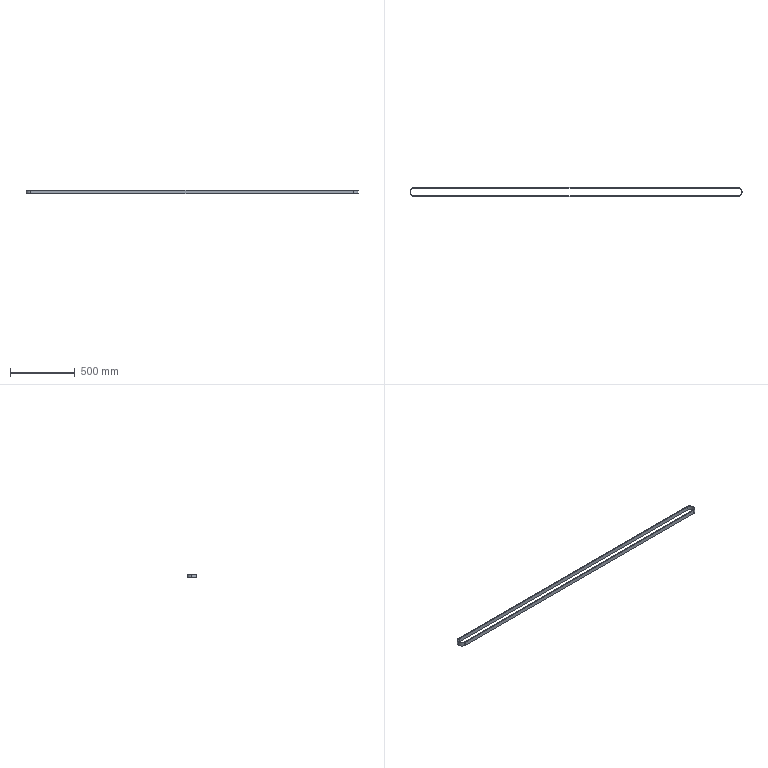Part | SolidWorks | features ExtruThin 1 | 1 solid | 12 faces | box 2564 x 70.66 x 30 mm | volume 701169 mm3 | cylinder 6 | plane 6 | commonest cylinder face diameters 61.66 x3 70.66 x3
STEP:
#1=CARTESIAN_POINT('',(-1246.5,30.83,30.));
#2=VERTEX_POINT('',#1);
#3=CARTESIAN_POINT('',(-1277.33,0.,30.));
#4=VERTEX_POINT('',#3);
#5=CARTESIAN_POINT('',(-1246.5,0.,30.));
#6=DIRECTION('',(0.,0.,1.));
#7=DIRECTION('',(1.,0.,0.));
#8=AXIS2_PLACEMENT_3D('',#5,#6,#7);
#9=CIRCLE('',#8,30.83);
#10=EDGE_CURVE('',#2,#4,#9,.T.);
#11=ORIENTED_EDGE('',*,*,#10,.T.);
#12=CARTESIAN_POINT('',(-1277.33,0.,0.));
#13=VERTEX_POINT('',#12);
#14=CARTESIAN_POINT('',(-1277.33,0.,30.));
#15=DIRECTION('',(0.,0.,-1.));
#16=VECTOR('',#15,1000.);
#17=LINE('',#14,#16);
#18=EDGE_CURVE('',#4,#13,#17,.T.);
#19=ORIENTED_EDGE('',*,*,#18,.T.);
#20=CARTESIAN_POINT('',(-1246.5,30.83,0.));
#21=VERTEX_POINT('',#20);
#22=CARTESIAN_POINT('',(-1246.5,0.,0.));
#23=DIRECTION('',(0.,0.,1.));
#24=DIRECTION('',(1.,0.,0.));
#25=AXIS2_PLACEMENT_3D('',#22,#23,#24);
#26=CIRCLE('',#25,30.83);
#27=EDGE_CURVE('',#21,#13,#26,.T.);
#28=ORIENTED_EDGE('',*,*,#27,.F.);
#29=CARTESIAN_POINT('',(-1246.5,30.83,30.));
#30=DIRECTION('',(0.,0.,-1.));
#31=VECTOR('',#30,1000.);
#32=LINE('',#29,#31);
#33=EDGE_CURVE('',#2,#21,#32,.T.);
#34=ORIENTED_EDGE('',*,*,#33,.F.);
#35=EDGE_LOOP('',(#11,#19,#28,#34));
#36=FACE_OUTER_BOUND('',#35,.T.);
#37=CARTESIAN_POINT('',(-1246.5,0.,30.));
#38=DIRECTION('',(0.,0.,-1.));
#39=DIRECTION('',(-1.,0.,0.));
#40=AXIS2_PLACEMENT_3D('',#37,#38,#39);
#41=CYLINDRICAL_SURFACE('',#40,30.83);
#42=ADVANCED_FACE('',(#36),#41,.F.);
#43=CARTESIAN_POINT('',(-1281.83,0.,30.));
#44=VERTEX_POINT('',#43);
#45=CARTESIAN_POINT('',(-1246.5,-35.33,30.));
#46=VERTEX_POINT('',#45);
#47=CARTESIAN_POINT('',(-1246.5,0.,30.));
#48=DIRECTION('',(0.,0.,1.));
#49=DIRECTION('',(1.,0.,0.));
#50=AXIS2_PLACEMENT_3D('',#47,#48,#49);
#51=CIRCLE('',#50,35.33);
#52=EDGE_CURVE('',#44,#46,#51,.T.);
#53=ORIENTED_EDGE('',*,*,#52,.F.);
#54=CARTESIAN_POINT('',(-1281.83,0.,0.));
#55=VERTEX_POINT('',#54);
#56=CARTESIAN_POINT('',(-1281.83,0.,30.));
#57=DIRECTION('',(0.,0.,-1.));
#58=VECTOR('',#57,1000.);
#59=LINE('',#56,#58);
#60=EDGE_CURVE('',#44,#55,#59,.T.);
#61=ORIENTED_EDGE('',*,*,#60,.T.);
#62=CARTESIAN_POINT('',(-1246.5,-35.33,0.));
#63=VERTEX_POINT('',#62);
#64=CARTESIAN_POINT('',(-1246.5,0.,0.));
#65=DIRECTION('',(0.,0.,1.));
#66=DIRECTION('',(1.,0.,0.));
#67=AXIS2_PLACEMENT_3D('',#64,#65,#66);
#68=CIRCLE('',#67,35.33);
#69=EDGE_CURVE('',#55,#63,#68,.T.);
#70=ORIENTED_EDGE('',*,*,#69,.T.);
#71=CARTESIAN_POINT('',(-1246.5,-35.33,30.));
#72=DIRECTION('',(0.,0.,-1.));
#73=VECTOR('',#72,1000.);
#74=LINE('',#71,#73);
#75=EDGE_CURVE('',#46,#63,#74,.T.);
#76=ORIENTED_EDGE('',*,*,#75,.F.);
#77=EDGE_LOOP('',(#53,#61,#70,#76));
#78=FACE_OUTER_BOUND('',#77,.T.);
#79=CARTESIAN_POINT('',(-1246.5,0.,30.));
#80=DIRECTION('',(0.,0.,-1.));
#81=DIRECTION('',(-1.,0.,0.));
#82=AXIS2_PLACEMENT_3D('',#79,#80,#81);
#83=CYLINDRICAL_SURFACE('',#82,35.33);
#84=ADVANCED_FACE('',(#78),#83,.T.);
#85=CARTESIAN_POINT('',(-1246.5,35.33,30.));
#86=VERTEX_POINT('',#85);
#87=CARTESIAN_POINT('',(-1246.5,0.,30.));
#88=DIRECTION('',(0.,0.,1.));
#89=DIRECTION('',(1.,0.,0.));
#90=AXIS2_PLACEMENT_3D('',#87,#88,#89);
#91=CIRCLE('',#90,35.33);
#92=EDGE_CURVE('',#86,#44,#91,.T.);
#93=ORIENTED_EDGE('',*,*,#92,.T.);
#94=ORIENTED_EDGE('',*,*,#52,.T.);
#95=CARTESIAN_POINT('',(1246.5,-35.33,30.));
#96=VERTEX_POINT('',#95);
#97=CARTESIAN_POINT('',(-1246.5,-35.33,30.));
#98=DIRECTION('',(1.,0.,0.));
#99=VECTOR('',#98,1000.);
#100=LINE('',#97,#99);
#101=EDGE_CURVE('',#46,#96,#100,.T.);
#102=ORIENTED_EDGE('',*,*,#101,.T.);
#103=CARTESIAN_POINT('',(1246.5,35.33,30.));
#104=VERTEX_POINT('',#103);
#105=CARTESIAN_POINT('',(1246.5,0.,30.));
#106=DIRECTION('',(0.,0.,1.));
#107=DIRECTION('',(1.,0.,0.));
#108=AXIS2_PLACEMENT_3D('',#105,#106,#107);
#109=CIRCLE('',#108,35.33);
#110=EDGE_CURVE('',#96,#104,#109,.T.);
#111=ORIENTED_EDGE('',*,*,#110,.T.);
#112=CARTESIAN_POINT('',(-1246.5,35.33,30.));
#113=DIRECTION('',(-1.,0.,0.));
#114=VECTOR('',#113,1000.);
#115=LINE('',#112,#114);
#116=EDGE_CURVE('',#104,#86,#115,.T.);
#117=ORIENTED_EDGE('',*,*,#116,.T.);
#118=EDGE_LOOP('',(#93,#94,#102,#111,#117));
#119=FACE_OUTER_BOUND('',#118,.T.);
#120=CARTESIAN_POINT('',(-1246.5,-30.83,30.));
#121=VERTEX_POINT('',#120);
#122=CARTESIAN_POINT('',(1246.5,-30.83,30.));
#123=VERTEX_POINT('',#122);
#124=CARTESIAN_POINT('',(-1246.5,-30.83,30.));
#125=DIRECTION('',(1.,0.,0.));
#126=VECTOR('',#125,1000.);
#127=LINE('',#124,#126);
#128=EDGE_CURVE('',#121,#123,#127,.T.);
#129=ORIENTED_EDGE('',*,*,#128,.F.);
#130=CARTESIAN_POINT('',(-1246.5,0.,30.));
#131=DIRECTION('',(0.,0.,1.));
#132=DIRECTION('',(1.,0.,0.));
#133=AXIS2_PLACEMENT_3D('',#130,#131,#132);
#134=CIRCLE('',#133,30.83);
#135=EDGE_CURVE('',#4,#121,#134,.T.);
#136=ORIENTED_EDGE('',*,*,#135,.F.);
#137=ORIENTED_EDGE('',*,*,#10,.F.);
#138=CARTESIAN_POINT('',(1246.5,30.83,30.));
#139=VERTEX_POINT('',#138);
#140=CARTESIAN_POINT('',(-1246.5,30.83,30.));
#141=DIRECTION('',(-1.,0.,0.));
#142=VECTOR('',#141,1000.);
#143=LINE('',#140,#142);
#144=EDGE_CURVE('',#139,#2,#143,.T.);
#145=ORIENTED_EDGE('',*,*,#144,.F.);
#146=CARTESIAN_POINT('',(1246.5,0.,30.));
#147=DIRECTION('',(0.,0.,1.));
#148=DIRECTION('',(1.,0.,0.));
#149=AXIS2_PLACEMENT_3D('',#146,#147,#148);
#150=CIRCLE('',#149,30.83);
#151=EDGE_CURVE('',#123,#139,#150,.T.);
#152=ORIENTED_EDGE('',*,*,#151,.F.);
#153=EDGE_LOOP('',(#129,#136,#137,#145,#152));
#154=FACE_BOUND('',#153,.T.);
#155=CARTESIAN_POINT('',(-1246.5,0.,30.));
#156=DIRECTION('',(0.,0.,1.));
#157=DIRECTION('',(1.,0.,0.));
#158=AXIS2_PLACEMENT_3D('',#155,#156,#157);
#159=PLANE('',#158);
#160=ADVANCED_FACE('',(#119,#154),#159,.T.);
#161=CARTESIAN_POINT('',(-1246.5,35.33,0.));
#162=VERTEX_POINT('',#161);
#163=CARTESIAN_POINT('',(-1246.5,0.,0.));
#164=DIRECTION('',(0.,0.,1.));
#165=DIRECTION('',(1.,0.,0.));
#166=AXIS2_PLACEMENT_3D('',#163,#164,#165);
#167=CIRCLE('',#166,35.33);
#168=EDGE_CURVE('',#162,#55,#167,.T.);
#169=ORIENTED_EDGE('',*,*,#168,.F.);
#170=CARTESIAN_POINT('',(1246.5,35.33,0.));
#171=VERTEX_POINT('',#170);
#172=CARTESIAN_POINT('',(-1246.5,35.33,0.));
#173=DIRECTION('',(-1.,0.,0.));
#174=VECTOR('',#173,1000.);
#175=LINE('',#172,#174);
#176=EDGE_CURVE('',#171,#162,#175,.T.);
#177=ORIENTED_EDGE('',*,*,#176,.F.);
#178=CARTESIAN_POINT('',(1246.5,-35.33,0.));
#179=VERTEX_POINT('',#178);
#180=CARTESIAN_POINT('',(1246.5,0.,0.));
#181=DIRECTION('',(0.,0.,1.));
#182=DIRECTION('',(1.,0.,0.));
#183=AXIS2_PLACEMENT_3D('',#180,#181,#182);
#184=CIRCLE('',#183,35.33);
#185=EDGE_CURVE('',#179,#171,#184,.T.);
#186=ORIENTED_EDGE('',*,*,#185,.F.);
#187=CARTESIAN_POINT('',(-1246.5,-35.33,0.));
#188=DIRECTION('',(1.,0.,0.));
#189=VECTOR('',#188,1000.);
#190=LINE('',#187,#189);
#191=EDGE_CURVE('',#63,#179,#190,.T.);
#192=ORIENTED_EDGE('',*,*,#191,.F.);
#193=ORIENTED_EDGE('',*,*,#69,.F.);
#194=EDGE_LOOP('',(#169,#177,#186,#192,#193));
#195=FACE_OUTER_BOUND('',#194,.T.);
#196=ORIENTED_EDGE('',*,*,#27,.T.);
#197=CARTESIAN_POINT('',(-1246.5,-30.83,0.));
#198=VERTEX_POINT('',#197);
#199=CARTESIAN_POINT('',(-1246.5,0.,0.));
#200=DIRECTION('',(0.,0.,1.));
#201=DIRECTION('',(1.,0.,0.));
#202=AXIS2_PLACEMENT_3D('',#199,#200,#201);
#203=CIRCLE('',#202,30.83);
#204=EDGE_CURVE('',#13,#198,#203,.T.);
#205=ORIENTED_EDGE('',*,*,#204,.T.);
#206=CARTESIAN_POINT('',(1246.5,-30.83,0.));
#207=VERTEX_POINT('',#206);
#208=CARTESIAN_POINT('',(-1246.5,-30.83,0.));
#209=DIRECTION('',(1.,0.,0.));
#210=VECTOR('',#209,1000.);
#211=LINE('',#208,#210);
#212=EDGE_CURVE('',#198,#207,#211,.T.);
#213=ORIENTED_EDGE('',*,*,#212,.T.);
#214=CARTESIAN_POINT('',(1246.5,30.83,0.));
#215=VERTEX_POINT('',#214);
#216=CARTESIAN_POINT('',(1246.5,0.,0.));
#217=DIRECTION('',(0.,0.,1.));
#218=DIRECTION('',(1.,0.,0.));
#219=AXIS2_PLACEMENT_3D('',#216,#217,#218);
#220=CIRCLE('',#219,30.83);
#221=EDGE_CURVE('',#207,#215,#220,.T.);
#222=ORIENTED_EDGE('',*,*,#221,.T.);
#223=CARTESIAN_POINT('',(-1246.5,30.83,0.));
#224=DIRECTION('',(-1.,0.,0.));
#225=VECTOR('',#224,1000.);
#226=LINE('',#223,#225);
#227=EDGE_CURVE('',#215,#21,#226,.T.);
#228=ORIENTED_EDGE('',*,*,#227,.T.);
#229=EDGE_LOOP('',(#196,#205,#213,#222,#228));
#230=FACE_BOUND('',#229,.T.);
#231=CARTESIAN_POINT('',(-1246.5,0.,0.));
#232=DIRECTION('',(0.,0.,1.));
#233=DIRECTION('',(1.,0.,0.));
#234=AXIS2_PLACEMENT_3D('',#231,#232,#233);
#235=PLANE('',#234);
#236=ADVANCED_FACE('',(#195,#230),#235,.F.);
#237=ORIENTED_EDGE('',*,*,#60,.F.);
#238=ORIENTED_EDGE('',*,*,#92,.F.);
#239=CARTESIAN_POINT('',(-1246.5,35.33,30.));
#240=DIRECTION('',(0.,0.,-1.));
#241=VECTOR('',#240,1000.);
#242=LINE('',#239,#241);
#243=EDGE_CURVE('',#86,#162,#242,.T.);
#244=ORIENTED_EDGE('',*,*,#243,.T.);
#245=ORIENTED_EDGE('',*,*,#168,.T.);
#246=EDGE_LOOP('',(#237,#238,#244,#245));
#247=FACE_OUTER_BOUND('',#246,.T.);
#248=CARTESIAN_POINT('',(-1246.5,0.,30.));
#249=DIRECTION('',(0.,0.,-1.));
#250=DIRECTION('',(-1.,0.,0.));
#251=AXIS2_PLACEMENT_3D('',#248,#249,#250);
#252=CYLINDRICAL_SURFACE('',#251,35.33);
#253=ADVANCED_FACE('',(#247),#252,.T.);
#254=ORIENTED_EDGE('',*,*,#191,.T.);
#255=CARTESIAN_POINT('',(1246.5,-35.33,30.));
#256=DIRECTION('',(0.,0.,-1.));
#257=VECTOR('',#256,1000.);
#258=LINE('',#255,#257);
#259=EDGE_CURVE('',#96,#179,#258,.T.);
#260=ORIENTED_EDGE('',*,*,#259,.F.);
#261=ORIENTED_EDGE('',*,*,#101,.F.);
#262=ORIENTED_EDGE('',*,*,#75,.T.);
#263=EDGE_LOOP('',(#254,#260,#261,#262));
#264=FACE_OUTER_BOUND('',#263,.T.);
#265=CARTESIAN_POINT('',(-1246.5,-35.33,30.));
#266=DIRECTION('',(0.,1.,0.));
#267=DIRECTION('',(0.,0.,1.));
#268=AXIS2_PLACEMENT_3D('',#265,#266,#267);
#269=PLANE('',#268);
#270=ADVANCED_FACE('',(#264),#269,.F.);
#271=ORIENTED_EDGE('',*,*,#185,.T.);
#272=CARTESIAN_POINT('',(1246.5,35.33,30.));
#273=DIRECTION('',(0.,0.,-1.));
#274=VECTOR('',#273,1000.);
#275=LINE('',#272,#274);
#276=EDGE_CURVE('',#104,#171,#275,.T.);
#277=ORIENTED_EDGE('',*,*,#276,.F.);
#278=ORIENTED_EDGE('',*,*,#110,.F.);
#279=ORIENTED_EDGE('',*,*,#259,.T.);
#280=EDGE_LOOP('',(#271,#277,#278,#279));
#281=FACE_OUTER_BOUND('',#280,.T.);
#282=CARTESIAN_POINT('',(1246.5,0.,30.));
#283=DIRECTION('',(0.,0.,-1.));
#284=DIRECTION('',(-1.,0.,0.));
#285=AXIS2_PLACEMENT_3D('',#282,#283,#284);
#286=CYLINDRICAL_SURFACE('',#285,35.33);
#287=ADVANCED_FACE('',(#281),#286,.T.);
#288=ORIENTED_EDGE('',*,*,#176,.T.);
#289=ORIENTED_EDGE('',*,*,#243,.F.);
#290=ORIENTED_EDGE('',*,*,#116,.F.);
#291=ORIENTED_EDGE('',*,*,#276,.T.);
#292=EDGE_LOOP('',(#288,#289,#290,#291));
#293=FACE_OUTER_BOUND('',#292,.T.);
#294=CARTESIAN_POINT('',(-1246.5,35.33,30.));
#295=DIRECTION('',(0.,-1.,0.));
#296=DIRECTION('',(0.,0.,-1.));
#297=AXIS2_PLACEMENT_3D('',#294,#295,#296);
#298=PLANE('',#297);
#299=ADVANCED_FACE('',(#293),#298,.F.);
#300=ORIENTED_EDGE('',*,*,#18,.F.);
#301=ORIENTED_EDGE('',*,*,#135,.T.);
#302=CARTESIAN_POINT('',(-1246.5,-30.83,30.));
#303=DIRECTION('',(0.,0.,-1.));
#304=VECTOR('',#303,1000.);
#305=LINE('',#302,#304);
#306=EDGE_CURVE('',#121,#198,#305,.T.);
#307=ORIENTED_EDGE('',*,*,#306,.T.);
#308=ORIENTED_EDGE('',*,*,#204,.F.);
#309=EDGE_LOOP('',(#300,#301,#307,#308));
#310=FACE_OUTER_BOUND('',#309,.T.);
#311=CARTESIAN_POINT('',(-1246.5,0.,30.));
#312=DIRECTION('',(0.,0.,-1.));
#313=DIRECTION('',(-1.,0.,0.));
#314=AXIS2_PLACEMENT_3D('',#311,#312,#313);
#315=CYLINDRICAL_SURFACE('',#314,30.83);
#316=ADVANCED_FACE('',(#310),#315,.F.);
#317=ORIENTED_EDGE('',*,*,#212,.F.);
#318=ORIENTED_EDGE('',*,*,#306,.F.);
#319=ORIENTED_EDGE('',*,*,#128,.T.);
#320=CARTESIAN_POINT('',(1246.5,-30.83,30.));
#321=DIRECTION('',(0.,0.,-1.));
#322=VECTOR('',#321,1000.);
#323=LINE('',#320,#322);
#324=EDGE_CURVE('',#123,#207,#323,.T.);
#325=ORIENTED_EDGE('',*,*,#324,.T.);
#326=EDGE_LOOP('',(#317,#318,#319,#325));
#327=FACE_OUTER_BOUND('',#326,.T.);
#328=CARTESIAN_POINT('',(-1246.5,-30.83,30.));
#329=DIRECTION('',(0.,1.,0.));
#330=DIRECTION('',(0.,0.,1.));
#331=AXIS2_PLACEMENT_3D('',#328,#329,#330);
#332=PLANE('',#331);
#333=ADVANCED_FACE('',(#327),#332,.T.);
#334=ORIENTED_EDGE('',*,*,#221,.F.);
#335=ORIENTED_EDGE('',*,*,#324,.F.);
#336=ORIENTED_EDGE('',*,*,#151,.T.);
#337=CARTESIAN_POINT('',(1246.5,30.83,30.));
#338=DIRECTION('',(0.,0.,-1.));
#339=VECTOR('',#338,1000.);
#340=LINE('',#337,#339);
#341=EDGE_CURVE('',#139,#215,#340,.T.);
#342=ORIENTED_EDGE('',*,*,#341,.T.);
#343=EDGE_LOOP('',(#334,#335,#336,#342));
#344=FACE_OUTER_BOUND('',#343,.T.);
#345=CARTESIAN_POINT('',(1246.5,0.,30.));
#346=DIRECTION('',(0.,0.,-1.));
#347=DIRECTION('',(-1.,0.,0.));
#348=AXIS2_PLACEMENT_3D('',#345,#346,#347);
#349=CYLINDRICAL_SURFACE('',#348,30.83);
#350=ADVANCED_FACE('',(#344),#349,.F.);
#351=ORIENTED_EDGE('',*,*,#227,.F.);
#352=ORIENTED_EDGE('',*,*,#341,.F.);
#353=ORIENTED_EDGE('',*,*,#144,.T.);
#354=ORIENTED_EDGE('',*,*,#33,.T.);
#355=EDGE_LOOP('',(#351,#352,#353,#354));
#356=FACE_OUTER_BOUND('',#355,.T.);
#357=CARTESIAN_POINT('',(-1246.5,30.83,30.));
#358=DIRECTION('',(0.,-1.,0.));
#359=DIRECTION('',(0.,0.,-1.));
#360=AXIS2_PLACEMENT_3D('',#357,#358,#359);
#361=PLANE('',#360);
#362=ADVANCED_FACE('',(#356),#361,.T.);
#363=CLOSED_SHELL('',(#42,#84,#160,#236,#253,#270,#287,#299,#316,#333,#350,#362));
#364=MANIFOLD_SOLID_BREP('',#363);
#365=CARTESIAN_POINT('',(0.,0.,0.));
#366=DIRECTION('',(0.,0.,1.));
#367=DIRECTION('',(1.,0.,0.));
#368=AXIS2_PLACEMENT_3D('',#365,#366,#367);
#369=(LENGTH_UNIT()NAMED_UNIT(*)SI_UNIT(.MILLI.,.METRE.));
#370=UNCERTAINTY_MEASURE_WITH_UNIT(LENGTH_MEASURE(0.00001),#369,'','');
#371=(NAMED_UNIT(*)PLANE_ANGLE_UNIT()SI_UNIT($,.RADIAN.));
#372=(NAMED_UNIT(*)SI_UNIT($,.STERADIAN.)SOLID_ANGLE_UNIT());
#373=(GEOMETRIC_REPRESENTATION_CONTEXT(3)GLOBAL_UNCERTAINTY_ASSIGNED_CONTEXT((#370))GLOBAL_UNIT_ASSIGNED_CONTEXT((#369,#371,#372))REPRESENTATION_CONTEXT('',''));
#374=ADVANCED_BREP_SHAPE_REPRESENTATION('',(#364,#368),#373);